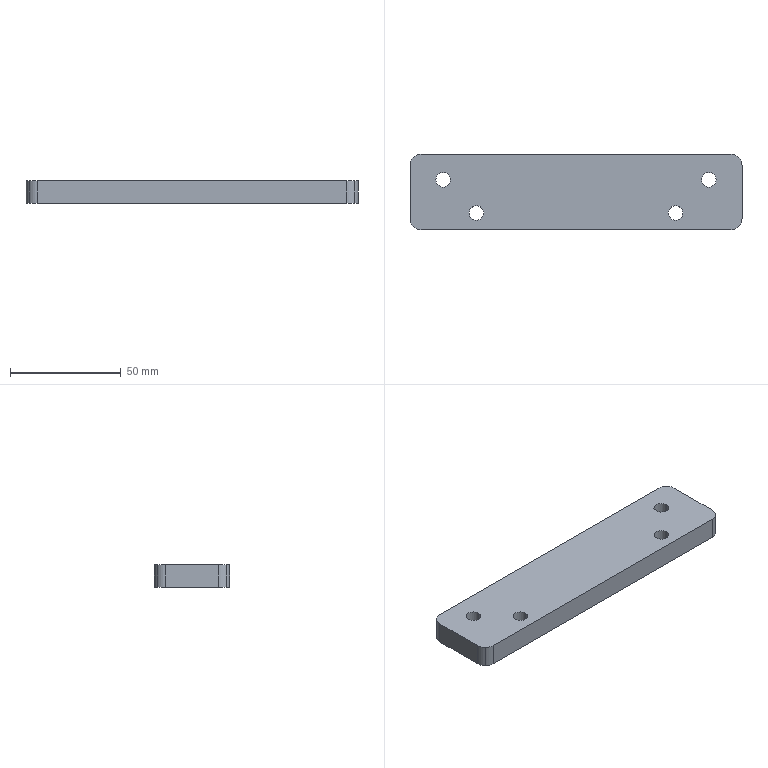Part | STEP file | DCV-000-012 | 1 solid | 22 faces | box 150 x 34 x 10 mm | volume 49407 mm3 | cylinder 16 | plane 6 | commonest cylinder face diameters 10 x8 6.6 x4 6.647 x4